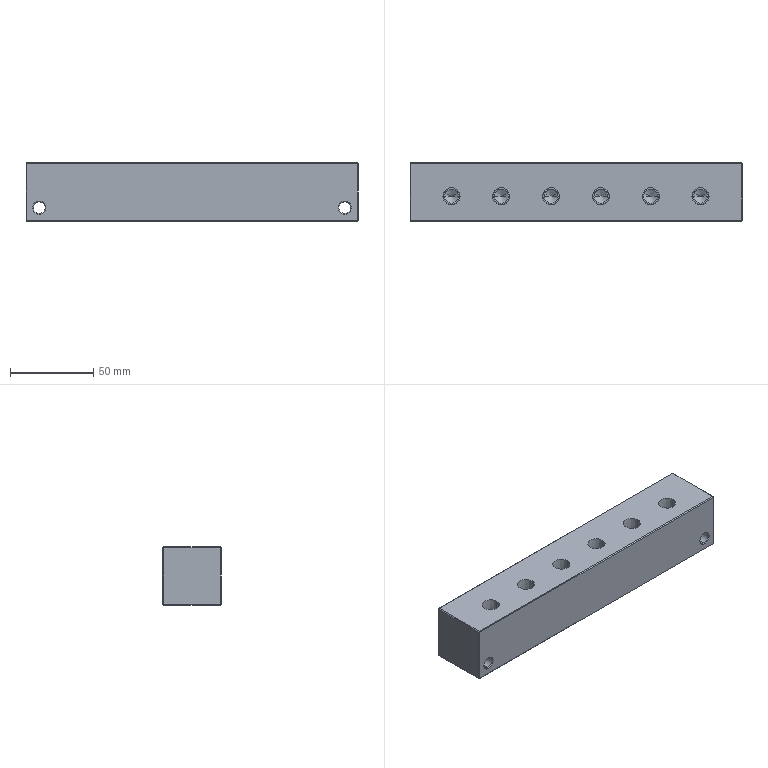Part | STEP file | OP10-136_junction block (F) | 1 solid | 122 faces | box 200 x 35 x 35 mm | volume 224966 mm3 | cone 44 | plane 40 | cylinder 38 | commonest cylinder face diameters 8.433 x30 7 x4 11 x4